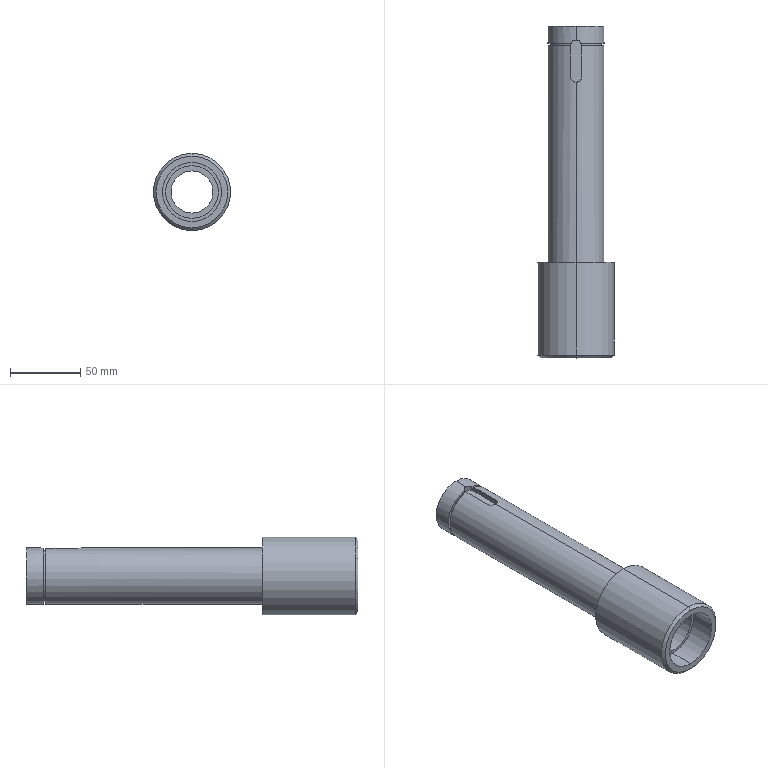Part | SolidWorks | features BaseBody 1 | 1 solid | 37 faces | box 55 x 236 x 55 mm | volume 172352 mm3 | cylinder 22 | plane 13 | cone 2 | commonest cylinder face diameters 40 x6 37.376 x4 8 x2 30 x2 36.4 x2 37 x2
STEP:
#1=CARTESIAN_POINT('',(4.,200.,19.596));
#2=VERTEX_POINT('',#1);
#3=CARTESIAN_POINT('',(0.,196.,20.));
#4=VERTEX_POINT('',#3);
#5=CARTESIAN_POINT('',(4.,200.,19.596));
#6=CARTESIAN_POINT('',(4.,199.735,19.596));
#7=CARTESIAN_POINT('',(3.974,199.475,19.601));
#8=CARTESIAN_POINT('',(3.872,198.963,19.622));
#9=CARTESIAN_POINT('',(3.795,198.709,19.637));
#10=CARTESIAN_POINT('',(3.594,198.225,19.675));
#11=CARTESIAN_POINT('',(3.471,197.996,19.697));
#12=CARTESIAN_POINT('',(3.181,197.561,19.746));
#13=CARTESIAN_POINT('',(3.013,197.356,19.773));
#14=CARTESIAN_POINT('',(2.645,196.989,19.825));
#15=CARTESIAN_POINT('',(2.445,196.823,19.851));
#16=CARTESIAN_POINT('',(2.008,196.531,19.9));
#17=CARTESIAN_POINT('',(1.777,196.407,19.922));
#18=CARTESIAN_POINT('',(1.296,196.207,19.959));
#19=CARTESIAN_POINT('',(1.044,196.13,19.974));
#20=CARTESIAN_POINT('',(0.5265,196.026,19.995));
#21=CARTESIAN_POINT('',(0.2648,196.,20.));
#22=CARTESIAN_POINT('',(0.,196.,20.));
#23=B_SPLINE_CURVE_WITH_KNOTS('',3,(#5,#6,#7,#8,#9,#10,#11,#12,#13,#14,#15,#16,#17,#18,#19,#20,#21,#22),.UNSPECIFIED.,.F.,.F.,(4,2,2,2,2,2,2,2,4),(0.,0.0007831,0.001566,0.002349,0.003132,0.003915,0.004698,0.005481,0.006264),.UNSPECIFIED.);
#24=EDGE_CURVE('',#2,#4,#23,.T.);
#25=ORIENTED_EDGE('',*,*,#24,.T.);
#26=CARTESIAN_POINT('',(0.,68.,20.));
#27=VERTEX_POINT('',#26);
#28=CARTESIAN_POINT('',(0.,236.,20.));
#29=DIRECTION('',(0.,-1.,0.));
#30=VECTOR('',#29,1000.);
#31=LINE('',#28,#30);
#32=EDGE_CURVE('',#4,#27,#31,.T.);
#33=ORIENTED_EDGE('',*,*,#32,.T.);
#34=CARTESIAN_POINT('',(0.,68.,-20.));
#35=VERTEX_POINT('',#34);
#36=CARTESIAN_POINT('',(0.,68.,0.));
#37=DIRECTION('',(0.,1.,0.));
#38=DIRECTION('',(0.,0.,-1.));
#39=AXIS2_PLACEMENT_3D('',#36,#37,#38);
#40=CIRCLE('',#39,20.);
#41=EDGE_CURVE('',#27,#35,#40,.T.);
#42=ORIENTED_EDGE('',*,*,#41,.T.);
#43=CARTESIAN_POINT('',(0.,222.,-20.));
#44=VERTEX_POINT('',#43);
#45=CARTESIAN_POINT('',(0.,236.,-20.));
#46=DIRECTION('',(0.,-1.,0.));
#47=VECTOR('',#46,1000.);
#48=LINE('',#45,#47);
#49=EDGE_CURVE('',#44,#35,#48,.T.);
#50=ORIENTED_EDGE('',*,*,#49,.F.);
#51=CARTESIAN_POINT('',(4.,222.,19.596));
#52=VERTEX_POINT('',#51);
#53=CARTESIAN_POINT('',(0.,222.,0.));
#54=DIRECTION('',(0.,-1.,0.));
#55=DIRECTION('',(0.,0.,-1.));
#56=AXIS2_PLACEMENT_3D('',#53,#54,#55);
#57=CIRCLE('',#56,20.);
#58=EDGE_CURVE('',#44,#52,#57,.T.);
#59=ORIENTED_EDGE('',*,*,#58,.T.);
#60=CARTESIAN_POINT('',(4.,236.,19.596));
#61=DIRECTION('',(0.,-1.,0.));
#62=VECTOR('',#61,1000.);
#63=LINE('',#60,#62);
#64=EDGE_CURVE('',#52,#2,#63,.T.);
#65=ORIENTED_EDGE('',*,*,#64,.T.);
#66=EDGE_LOOP('',(#25,#33,#42,#50,#59,#65));
#67=FACE_OUTER_BOUND('',#66,.T.);
#68=CARTESIAN_POINT('',(0.,236.,0.));
#69=DIRECTION('',(0.,-1.,0.));
#70=DIRECTION('',(0.,0.,-1.));
#71=AXIS2_PLACEMENT_3D('',#68,#69,#70);
#72=CYLINDRICAL_SURFACE('',#71,20.);
#73=ADVANCED_FACE('',(#67),#72,.T.);
#74=CARTESIAN_POINT('',(-3.666,223.6,17.827));
#75=VERTEX_POINT('',#74);
#76=CARTESIAN_POINT('',(0.,223.6,-18.2));
#77=VERTEX_POINT('',#76);
#78=CARTESIAN_POINT('',(0.,223.6,0.));
#79=DIRECTION('',(0.,-1.,0.));
#80=DIRECTION('',(0.,0.,-1.));
#81=AXIS2_PLACEMENT_3D('',#78,#79,#80);
#82=CIRCLE('',#81,18.2);
#83=EDGE_CURVE('',#75,#77,#82,.T.);
#84=ORIENTED_EDGE('',*,*,#83,.T.);
#85=CARTESIAN_POINT('',(0.,222.,-18.2));
#86=VERTEX_POINT('',#85);
#87=CARTESIAN_POINT('',(0.,223.6,-18.2));
#88=DIRECTION('',(0.,-1.,0.));
#89=VECTOR('',#88,1000.);
#90=LINE('',#87,#89);
#91=EDGE_CURVE('',#77,#86,#90,.T.);
#92=ORIENTED_EDGE('',*,*,#91,.T.);
#93=CARTESIAN_POINT('',(-4.,222.,17.755));
#94=VERTEX_POINT('',#93);
#95=CARTESIAN_POINT('',(0.,222.,0.));
#96=DIRECTION('',(0.,-1.,0.));
#97=DIRECTION('',(0.,0.,-1.));
#98=AXIS2_PLACEMENT_3D('',#95,#96,#97);
#99=CIRCLE('',#98,18.2);
#100=EDGE_CURVE('',#94,#86,#99,.T.);
#101=ORIENTED_EDGE('',*,*,#100,.F.);
#102=CARTESIAN_POINT('',(-4.,222.,17.755));
#103=CARTESIAN_POINT('',(-4.,222.277,17.755));
#104=CARTESIAN_POINT('',(-3.972,222.549,17.761));
#105=CARTESIAN_POINT('',(-3.86,223.083,17.786));
#106=CARTESIAN_POINT('',(-3.776,223.347,17.804));
#107=CARTESIAN_POINT('',(-3.666,223.6,17.827));
#108=B_SPLINE_CURVE_WITH_KNOTS('',3,(#102,#103,#104,#105,#106,#107),.UNSPECIFIED.,.F.,.F.,(4,2,4),(0.,0.0008187,0.001637),.UNSPECIFIED.);
#109=EDGE_CURVE('',#94,#75,#108,.T.);
#110=ORIENTED_EDGE('',*,*,#109,.T.);
#111=EDGE_LOOP('',(#84,#92,#101,#110));
#112=FACE_OUTER_BOUND('',#111,.T.);
#113=CARTESIAN_POINT('',(0.,223.6,0.));
#114=DIRECTION('',(0.,-1.,0.));
#115=DIRECTION('',(0.,0.,-1.));
#116=AXIS2_PLACEMENT_3D('',#113,#114,#115);
#117=CYLINDRICAL_SURFACE('',#116,18.2);
#118=ADVANCED_FACE('',(#112),#117,.T.);
#119=CARTESIAN_POINT('',(0.,68.,27.5));
#120=VERTEX_POINT('',#119);
#121=CARTESIAN_POINT('',(0.,68.,-27.5));
#122=VERTEX_POINT('',#121);
#123=CARTESIAN_POINT('',(0.,68.,0.));
#124=DIRECTION('',(0.,1.,0.));
#125=DIRECTION('',(0.,0.,-1.));
#126=AXIS2_PLACEMENT_3D('',#123,#124,#125);
#127=CIRCLE('',#126,27.5);
#128=EDGE_CURVE('',#120,#122,#127,.T.);
#129=ORIENTED_EDGE('',*,*,#128,.F.);
#130=CARTESIAN_POINT('',(0.,2.,27.5));
#131=VERTEX_POINT('',#130);
#132=CARTESIAN_POINT('',(0.,68.,27.5));
#133=DIRECTION('',(0.,-1.,0.));
#134=VECTOR('',#133,1000.);
#135=LINE('',#132,#134);
#136=EDGE_CURVE('',#120,#131,#135,.T.);
#137=ORIENTED_EDGE('',*,*,#136,.T.);
#138=CARTESIAN_POINT('',(0.,2.,-27.5));
#139=VERTEX_POINT('',#138);
#140=CARTESIAN_POINT('',(0.,2.,0.));
#141=DIRECTION('',(0.,1.,0.));
#142=DIRECTION('',(0.,0.,-1.));
#143=AXIS2_PLACEMENT_3D('',#140,#141,#142);
#144=CIRCLE('',#143,27.5);
#145=EDGE_CURVE('',#131,#139,#144,.T.);
#146=ORIENTED_EDGE('',*,*,#145,.T.);
#147=CARTESIAN_POINT('',(0.,68.,-27.5));
#148=DIRECTION('',(0.,-1.,0.));
#149=VECTOR('',#148,1000.);
#150=LINE('',#147,#149);
#151=EDGE_CURVE('',#122,#139,#150,.T.);
#152=ORIENTED_EDGE('',*,*,#151,.F.);
#153=EDGE_LOOP('',(#129,#137,#146,#152));
#154=FACE_OUTER_BOUND('',#153,.T.);
#155=CARTESIAN_POINT('',(0.,68.,0.));
#156=DIRECTION('',(0.,-1.,0.));
#157=DIRECTION('',(0.,0.,-1.));
#158=AXIS2_PLACEMENT_3D('',#155,#156,#157);
#159=CYLINDRICAL_SURFACE('',#158,27.5);
#160=ADVANCED_FACE('',(#154),#159,.T.);
#161=CARTESIAN_POINT('',(0.,236.,-20.));
#162=VERTEX_POINT('',#161);
#163=CARTESIAN_POINT('',(0.,236.,20.));
#164=VERTEX_POINT('',#163);
#165=CARTESIAN_POINT('',(0.,236.,0.));
#166=DIRECTION('',(0.,-1.,0.));
#167=DIRECTION('',(0.,0.,-1.));
#168=AXIS2_PLACEMENT_3D('',#165,#166,#167);
#169=CIRCLE('',#168,20.);
#170=EDGE_CURVE('',#162,#164,#169,.T.);
#171=ORIENTED_EDGE('',*,*,#170,.T.);
#172=CARTESIAN_POINT('',(0.,226.,20.));
#173=VERTEX_POINT('',#172);
#174=CARTESIAN_POINT('',(0.,236.,20.));
#175=DIRECTION('',(0.,-1.,0.));
#176=VECTOR('',#175,1000.);
#177=LINE('',#174,#176);
#178=EDGE_CURVE('',#164,#173,#177,.T.);
#179=ORIENTED_EDGE('',*,*,#178,.T.);
#180=CARTESIAN_POINT('',(3.666,223.6,19.661));
#181=VERTEX_POINT('',#180);
#182=CARTESIAN_POINT('',(0.,226.,20.));
#183=CARTESIAN_POINT('',(0.391,226.,20.));
#184=CARTESIAN_POINT('',(0.7721,225.944,19.989));
#185=CARTESIAN_POINT('',(1.33,225.778,19.957));
#186=CARTESIAN_POINT('',(1.513,225.708,19.943));
#187=CARTESIAN_POINT('',(1.862,225.546,19.914));
#188=CARTESIAN_POINT('',(2.03,225.452,19.897));
#189=CARTESIAN_POINT('',(2.352,225.241,19.862));
#190=CARTESIAN_POINT('',(2.507,225.123,19.843));
#191=CARTESIAN_POINT('',(2.796,224.867,19.804));
#192=CARTESIAN_POINT('',(2.93,224.73,19.785));
#193=CARTESIAN_POINT('',(3.302,224.29,19.727));
#194=CARTESIAN_POINT('',(3.51,223.957,19.69));
#195=CARTESIAN_POINT('',(3.666,223.6,19.661));
#196=B_SPLINE_CURVE_WITH_KNOTS('',3,(#182,#183,#184,#185,#186,#187,#188,#189,#190,#191,#192,#193,#194,#195),.UNSPECIFIED.,.F.,.F.,(4,2,2,2,2,2,4),(0.,0.001156,0.001734,0.002312,0.00289,0.003468,0.004624),.UNSPECIFIED.);
#197=EDGE_CURVE('',#173,#181,#196,.T.);
#198=ORIENTED_EDGE('',*,*,#197,.T.);
#199=CARTESIAN_POINT('',(0.,223.6,-20.));
#200=VERTEX_POINT('',#199);
#201=CARTESIAN_POINT('',(0.,223.6,0.));
#202=DIRECTION('',(0.,1.,0.));
#203=DIRECTION('',(0.,0.,-1.));
#204=AXIS2_PLACEMENT_3D('',#201,#202,#203);
#205=CIRCLE('',#204,20.);
#206=EDGE_CURVE('',#181,#200,#205,.T.);
#207=ORIENTED_EDGE('',*,*,#206,.T.);
#208=CARTESIAN_POINT('',(0.,236.,-20.));
#209=DIRECTION('',(0.,-1.,0.));
#210=VECTOR('',#209,1000.);
#211=LINE('',#208,#210);
#212=EDGE_CURVE('',#162,#200,#211,.T.);
#213=ORIENTED_EDGE('',*,*,#212,.F.);
#214=EDGE_LOOP('',(#171,#179,#198,#207,#213));
#215=FACE_OUTER_BOUND('',#214,.T.);
#216=CARTESIAN_POINT('',(0.,236.,0.));
#217=DIRECTION('',(0.,-1.,0.));
#218=DIRECTION('',(0.,0.,-1.));
#219=AXIS2_PLACEMENT_3D('',#216,#217,#218);
#220=CYLINDRICAL_SURFACE('',#219,20.);
#221=ADVANCED_FACE('',(#215),#220,.T.);
#222=CARTESIAN_POINT('',(0.,0.,25.5));
#223=VERTEX_POINT('',#222);
#224=CARTESIAN_POINT('',(0.,0.,-25.5));
#225=VERTEX_POINT('',#224);
#226=CARTESIAN_POINT('',(0.,0.,0.));
#227=DIRECTION('',(0.,1.,0.));
#228=DIRECTION('',(0.,0.,1.));
#229=AXIS2_PLACEMENT_3D('',#226,#227,#228);
#230=CIRCLE('',#229,25.5);
#231=EDGE_CURVE('',#223,#225,#230,.T.);
#232=ORIENTED_EDGE('',*,*,#231,.T.);
#233=CARTESIAN_POINT('',(0.,2.,-27.5));
#234=DIRECTION('',(0.,0.7071,-0.7071));
#235=VECTOR('',#234,1000.);
#236=LINE('',#233,#235);
#237=EDGE_CURVE('',#225,#139,#236,.T.);
#238=ORIENTED_EDGE('',*,*,#237,.T.);
#239=ORIENTED_EDGE('',*,*,#145,.F.);
#240=CARTESIAN_POINT('',(0.,2.,27.5));
#241=DIRECTION('',(0.,0.7071,0.7071));
#242=VECTOR('',#241,1000.);
#243=LINE('',#240,#242);
#244=EDGE_CURVE('',#223,#131,#243,.T.);
#245=ORIENTED_EDGE('',*,*,#244,.F.);
#246=EDGE_LOOP('',(#232,#238,#239,#245));
#247=FACE_OUTER_BOUND('',#246,.T.);
#248=CARTESIAN_POINT('',(0.,2.,0.));
#249=DIRECTION('',(0.,1.,0.));
#250=DIRECTION('',(0.,0.,1.));
#251=AXIS2_PLACEMENT_3D('',#248,#249,#250);
#252=CONICAL_SURFACE('',#251,27.5,0.7854);
#253=ADVANCED_FACE('',(#247),#252,.T.);
#254=CARTESIAN_POINT('',(0.,226.5,-18.5));
#255=VERTEX_POINT('',#254);
#256=CARTESIAN_POINT('',(0.,226.5,18.5));
#257=VERTEX_POINT('',#256);
#258=CARTESIAN_POINT('',(0.,226.5,0.));
#259=DIRECTION('',(0.,1.,0.));
#260=DIRECTION('',(0.,0.,1.));
#261=AXIS2_PLACEMENT_3D('',#258,#259,#260);
#262=CIRCLE('',#261,18.5);
#263=EDGE_CURVE('',#255,#257,#262,.T.);
#264=ORIENTED_EDGE('',*,*,#263,.F.);
#265=CARTESIAN_POINT('',(0.,236.,-18.5));
#266=VERTEX_POINT('',#265);
#267=CARTESIAN_POINT('',(0.,226.5,-18.5));
#268=DIRECTION('',(0.,1.,0.));
#269=VECTOR('',#268,1000.);
#270=LINE('',#267,#269);
#271=EDGE_CURVE('',#255,#266,#270,.T.);
#272=ORIENTED_EDGE('',*,*,#271,.T.);
#273=CARTESIAN_POINT('',(0.,236.,18.5));
#274=VERTEX_POINT('',#273);
#275=CARTESIAN_POINT('',(0.,236.,0.));
#276=DIRECTION('',(0.,-1.,0.));
#277=DIRECTION('',(0.,0.,1.));
#278=AXIS2_PLACEMENT_3D('',#275,#276,#277);
#279=CIRCLE('',#278,18.5);
#280=EDGE_CURVE('',#274,#266,#279,.T.);
#281=ORIENTED_EDGE('',*,*,#280,.F.);
#282=CARTESIAN_POINT('',(0.,226.5,18.5));
#283=DIRECTION('',(0.,1.,0.));
#284=VECTOR('',#283,1000.);
#285=LINE('',#282,#284);
#286=EDGE_CURVE('',#257,#274,#285,.T.);
#287=ORIENTED_EDGE('',*,*,#286,.F.);
#288=EDGE_LOOP('',(#264,#272,#281,#287));
#289=FACE_OUTER_BOUND('',#288,.T.);
#290=CARTESIAN_POINT('',(0.,226.5,0.));
#291=DIRECTION('',(0.,1.,0.));
#292=DIRECTION('',(0.,0.,1.));
#293=AXIS2_PLACEMENT_3D('',#290,#291,#292);
#294=CYLINDRICAL_SURFACE('',#293,18.5);
#295=ADVANCED_FACE('',(#289),#294,.F.);
#296=CARTESIAN_POINT('',(0.,18.,21.));
#297=VERTEX_POINT('',#296);
#298=CARTESIAN_POINT('',(0.,18.,-21.));
#299=VERTEX_POINT('',#298);
#300=CARTESIAN_POINT('',(0.,18.,0.));
#301=DIRECTION('',(0.,-1.,0.));
#302=DIRECTION('',(0.,0.,-1.));
#303=AXIS2_PLACEMENT_3D('',#300,#301,#302);
#304=CIRCLE('',#303,21.);
#305=EDGE_CURVE('',#297,#299,#304,.T.);
#306=ORIENTED_EDGE('',*,*,#305,.F.);
#307=CARTESIAN_POINT('',(0.,0.,21.));
#308=VERTEX_POINT('',#307);
#309=CARTESIAN_POINT('',(0.,18.,21.));
#310=DIRECTION('',(0.,-1.,0.));
#311=VECTOR('',#310,1000.);
#312=LINE('',#309,#311);
#313=EDGE_CURVE('',#297,#308,#312,.T.);
#314=ORIENTED_EDGE('',*,*,#313,.T.);
#315=CARTESIAN_POINT('',(0.,0.,-21.));
#316=VERTEX_POINT('',#315);
#317=CARTESIAN_POINT('',(0.,0.,0.));
#318=DIRECTION('',(0.,-1.,0.));
#319=DIRECTION('',(0.,0.,-1.));
#320=AXIS2_PLACEMENT_3D('',#317,#318,#319);
#321=CIRCLE('',#320,21.);
#322=EDGE_CURVE('',#308,#316,#321,.T.);
#323=ORIENTED_EDGE('',*,*,#322,.T.);
#324=CARTESIAN_POINT('',(0.,18.,-21.));
#325=DIRECTION('',(0.,-1.,0.));
#326=VECTOR('',#325,1000.);
#327=LINE('',#324,#326);
#328=EDGE_CURVE('',#299,#316,#327,.T.);
#329=ORIENTED_EDGE('',*,*,#328,.F.);
#330=EDGE_LOOP('',(#306,#314,#323,#329));
#331=FACE_OUTER_BOUND('',#330,.T.);
#332=CARTESIAN_POINT('',(0.,18.,0.));
#333=DIRECTION('',(0.,-1.,0.));
#334=DIRECTION('',(0.,0.,-1.));
#335=AXIS2_PLACEMENT_3D('',#332,#333,#334);
#336=CYLINDRICAL_SURFACE('',#335,21.);
#337=ADVANCED_FACE('',(#331),#336,.F.);
#338=CARTESIAN_POINT('',(0.,226.5,15.));
#339=VERTEX_POINT('',#338);
#340=CARTESIAN_POINT('',(0.,226.5,-15.));
#341=VERTEX_POINT('',#340);
#342=CARTESIAN_POINT('',(0.,226.5,0.));
#343=DIRECTION('',(0.,-1.,0.));
#344=DIRECTION('',(0.,0.,-1.));
#345=AXIS2_PLACEMENT_3D('',#342,#343,#344);
#346=CIRCLE('',#345,15.);
#347=EDGE_CURVE('',#339,#341,#346,.T.);
#348=ORIENTED_EDGE('',*,*,#347,.F.);
#349=CARTESIAN_POINT('',(0.,58.,15.));
#350=VERTEX_POINT('',#349);
#351=CARTESIAN_POINT('',(0.,68.,15.));
#352=DIRECTION('',(0.,-1.,0.));
#353=VECTOR('',#352,1000.);
#354=LINE('',#351,#353);
#355=EDGE_CURVE('',#339,#350,#354,.T.);
#356=ORIENTED_EDGE('',*,*,#355,.T.);
#357=CARTESIAN_POINT('',(0.,58.,-15.));
#358=VERTEX_POINT('',#357);
#359=CARTESIAN_POINT('',(0.,58.,0.));
#360=DIRECTION('',(0.,1.,0.));
#361=DIRECTION('',(0.,0.,-1.));
#362=AXIS2_PLACEMENT_3D('',#359,#360,#361);
#363=CIRCLE('',#362,15.);
#364=EDGE_CURVE('',#358,#350,#363,.T.);
#365=ORIENTED_EDGE('',*,*,#364,.F.);
#366=CARTESIAN_POINT('',(0.,68.,-15.));
#367=DIRECTION('',(0.,-1.,0.));
#368=VECTOR('',#367,1000.);
#369=LINE('',#366,#368);
#370=EDGE_CURVE('',#341,#358,#369,.T.);
#371=ORIENTED_EDGE('',*,*,#370,.F.);
#372=EDGE_LOOP('',(#348,#356,#365,#371));
#373=FACE_OUTER_BOUND('',#372,.T.);
#374=CARTESIAN_POINT('',(0.,68.,0.));
#375=DIRECTION('',(0.,-1.,0.));
#376=DIRECTION('',(0.,0.,-1.));
#377=AXIS2_PLACEMENT_3D('',#374,#375,#376);
#378=CYLINDRICAL_SURFACE('',#377,15.);
#379=ADVANCED_FACE('',(#373),#378,.F.);
#380=CARTESIAN_POINT('',(0.,48.,18.688));
#381=VERTEX_POINT('',#380);
#382=CARTESIAN_POINT('',(0.,48.,-18.688));
#383=VERTEX_POINT('',#382);
#384=CARTESIAN_POINT('',(0.,48.,0.));
#385=DIRECTION('',(0.,-1.,0.));
#386=DIRECTION('',(0.,0.,-1.));
#387=AXIS2_PLACEMENT_3D('',#384,#385,#386);
#388=CIRCLE('',#387,18.688);
#389=EDGE_CURVE('',#381,#383,#388,.T.);
#390=ORIENTED_EDGE('',*,*,#389,.F.);
#391=CARTESIAN_POINT('',(0.,18.,18.688));
#392=VERTEX_POINT('',#391);
#393=CARTESIAN_POINT('',(0.,58.,18.688));
#394=DIRECTION('',(0.,-1.,0.));
#395=VECTOR('',#394,1000.);
#396=LINE('',#393,#395);
#397=EDGE_CURVE('',#381,#392,#396,.T.);
#398=ORIENTED_EDGE('',*,*,#397,.T.);
#399=CARTESIAN_POINT('',(0.,18.,-18.688));
#400=VERTEX_POINT('',#399);
#401=CARTESIAN_POINT('',(0.,18.,0.));
#402=DIRECTION('',(0.,1.,0.));
#403=DIRECTION('',(0.,0.,-1.));
#404=AXIS2_PLACEMENT_3D('',#401,#402,#403);
#405=CIRCLE('',#404,18.688);
#406=EDGE_CURVE('',#400,#392,#405,.T.);
#407=ORIENTED_EDGE('',*,*,#406,.F.);
#408=CARTESIAN_POINT('',(0.,58.,-18.688));
#409=DIRECTION('',(0.,-1.,0.));
#410=VECTOR('',#409,1000.);
#411=LINE('',#408,#410);
#412=EDGE_CURVE('',#383,#400,#411,.T.);
#413=ORIENTED_EDGE('',*,*,#412,.F.);
#414=EDGE_LOOP('',(#390,#398,#407,#413));
#415=FACE_OUTER_BOUND('',#414,.T.);
#416=CARTESIAN_POINT('',(0.,58.,0.));
#417=DIRECTION('',(0.,-1.,0.));
#418=DIRECTION('',(0.,0.,-1.));
#419=AXIS2_PLACEMENT_3D('',#416,#417,#418);
#420=CYLINDRICAL_SURFACE('',#419,18.688);
#421=ADVANCED_FACE('',(#415),#420,.F.);
#422=CARTESIAN_POINT('',(0.,58.,18.688));
#423=VERTEX_POINT('',#422);
#424=CARTESIAN_POINT('',(0.,58.,-18.688));
#425=VERTEX_POINT('',#424);
#426=CARTESIAN_POINT('',(0.,58.,0.));
#427=DIRECTION('',(0.,-1.,0.));
#428=DIRECTION('',(0.,0.,-1.));
#429=AXIS2_PLACEMENT_3D('',#426,#427,#428);
#430=CIRCLE('',#429,18.688);
#431=EDGE_CURVE('',#423,#425,#430,.T.);
#432=ORIENTED_EDGE('',*,*,#431,.F.);
#433=CARTESIAN_POINT('',(0.,52.,18.688));
#434=VERTEX_POINT('',#433);
#435=CARTESIAN_POINT('',(0.,58.,18.688));
#436=DIRECTION('',(0.,-1.,0.));
#437=VECTOR('',#436,1000.);
#438=LINE('',#435,#437);
#439=EDGE_CURVE('',#423,#434,#438,.T.);
#440=ORIENTED_EDGE('',*,*,#439,.T.);
#441=CARTESIAN_POINT('',(0.,52.,-18.688));
#442=VERTEX_POINT('',#441);
#443=CARTESIAN_POINT('',(0.,52.,0.));
#444=DIRECTION('',(0.,1.,0.));
#445=DIRECTION('',(0.,0.,-1.));
#446=AXIS2_PLACEMENT_3D('',#443,#444,#445);
#447=CIRCLE('',#446,18.688);
#448=EDGE_CURVE('',#442,#434,#447,.T.);
#449=ORIENTED_EDGE('',*,*,#448,.F.);
#450=CARTESIAN_POINT('',(0.,58.,-18.688));
#451=DIRECTION('',(0.,-1.,0.));
#452=VECTOR('',#451,1000.);
#453=LINE('',#450,#452);
#454=EDGE_CURVE('',#425,#442,#453,.T.);
#455=ORIENTED_EDGE('',*,*,#454,.F.);
#456=EDGE_LOOP('',(#432,#440,#449,#455));
#457=FACE_OUTER_BOUND('',#456,.T.);
#458=CARTESIAN_POINT('',(0.,58.,0.));
#459=DIRECTION('',(0.,-1.,0.));
#460=DIRECTION('',(0.,0.,-1.));
#461=AXIS2_PLACEMENT_3D('',#458,#459,#460);
#462=CYLINDRICAL_SURFACE('',#461,18.688);
#463=ADVANCED_FACE('',(#457),#462,.F.);
#464=CARTESIAN_POINT('',(0.,52.,20.));
#465=VERTEX_POINT('',#464);
#466=CARTESIAN_POINT('',(0.,52.,-20.));
#467=VERTEX_POINT('',#466);
#468=CARTESIAN_POINT('',(0.,52.,0.));
#469=DIRECTION('',(0.,-1.,0.));
#470=DIRECTION('',(0.,0.,-1.));
#471=AXIS2_PLACEMENT_3D('',#468,#469,#470);
#472=CIRCLE('',#471,20.);
#473=EDGE_CURVE('',#465,#467,#472,.T.);
#474=ORIENTED_EDGE('',*,*,#473,.F.);
#475=CARTESIAN_POINT('',(0.,48.,20.));
#476=VERTEX_POINT('',#475);
#477=CARTESIAN_POINT('',(0.,52.,20.));
#478=DIRECTION('',(0.,-1.,0.));
#479=VECTOR('',#478,1000.);
#480=LINE('',#477,#479);
#481=EDGE_CURVE('',#465,#476,#480,.T.);
#482=ORIENTED_EDGE('',*,*,#481,.T.);
#483=CARTESIAN_POINT('',(0.,48.,-20.));
#484=VERTEX_POINT('',#483);
#485=CARTESIAN_POINT('',(0.,48.,0.));
#486=DIRECTION('',(0.,-1.,0.));
#487=DIRECTION('',(0.,0.,-1.));
#488=AXIS2_PLACEMENT_3D('',#485,#486,#487);
#489=CIRCLE('',#488,20.);
#490=EDGE_CURVE('',#476,#484,#489,.T.);
#491=ORIENTED_EDGE('',*,*,#490,.T.);
#492=CARTESIAN_POINT('',(0.,52.,-20.));
#493=DIRECTION('',(0.,-1.,0.));
#494=VECTOR('',#493,1000.);
#495=LINE('',#492,#494);
#496=EDGE_CURVE('',#467,#484,#495,.T.);
#497=ORIENTED_EDGE('',*,*,#496,.F.);
#498=EDGE_LOOP('',(#474,#482,#491,#497));
#499=FACE_OUTER_BOUND('',#498,.T.);
#500=CARTESIAN_POINT('',(0.,52.,0.));
#501=DIRECTION('',(0.,-1.,0.));
#502=DIRECTION('',(0.,0.,-1.));
#503=AXIS2_PLACEMENT_3D('',#500,#501,#502);
#504=CYLINDRICAL_SURFACE('',#503,20.);
#505=ADVANCED_FACE('',(#499),#504,.F.);
#506=ORIENTED_EDGE('',*,*,#32,.F.);
#507=CARTESIAN_POINT('',(-4.,200.,19.596));
#508=VERTEX_POINT('',#507);
#509=CARTESIAN_POINT('',(0.,196.,20.));
#510=CARTESIAN_POINT('',(-0.2648,196.,20.));
#511=CARTESIAN_POINT('',(-0.5251,196.026,19.995));
#512=CARTESIAN_POINT('',(-1.037,196.128,19.975));
#513=CARTESIAN_POINT('',(-1.291,196.205,19.96));
#514=CARTESIAN_POINT('',(-1.775,196.406,19.923));
#515=CARTESIAN_POINT('',(-2.005,196.529,19.9));
#516=CARTESIAN_POINT('',(-2.439,196.819,19.852));
#517=CARTESIAN_POINT('',(-2.644,196.987,19.825));
#518=CARTESIAN_POINT('',(-3.012,197.355,19.773));
#519=CARTESIAN_POINT('',(-3.177,197.555,19.747));
#520=CARTESIAN_POINT('',(-3.469,197.992,19.697));
#521=CARTESIAN_POINT('',(-3.593,198.223,19.675));
#522=CARTESIAN_POINT('',(-3.793,198.704,19.637));
#523=CARTESIAN_POINT('',(-3.87,198.956,19.622));
#524=CARTESIAN_POINT('',(-3.974,199.473,19.601));
#525=CARTESIAN_POINT('',(-4.,199.735,19.596));
#526=CARTESIAN_POINT('',(-4.,200.,19.596));
#527=B_SPLINE_CURVE_WITH_KNOTS('',3,(#509,#510,#511,#512,#513,#514,#515,#516,#517,#518,#519,#520,#521,#522,#523,#524,#525,#526),.UNSPECIFIED.,.F.,.F.,(4,2,2,2,2,2,2,2,4),(0.006264,0.007048,0.007831,0.008614,0.009397,0.01018,0.01096,0.01175,0.01253),.UNSPECIFIED.);
#528=EDGE_CURVE('',#4,#508,#527,.T.);
#529=ORIENTED_EDGE('',*,*,#528,.T.);
#530=CARTESIAN_POINT('',(-4.,222.,19.596));
#531=VERTEX_POINT('',#530);
#532=CARTESIAN_POINT('',(-4.,236.,19.596));
#533=DIRECTION('',(0.,1.,0.));
#534=VECTOR('',#533,1000.);
#535=LINE('',#532,#534);
#536=EDGE_CURVE('',#508,#531,#535,.T.);
#537=ORIENTED_EDGE('',*,*,#536,.T.);
#538=CARTESIAN_POINT('',(0.,222.,0.));
#539=DIRECTION('',(0.,-1.,0.));
#540=DIRECTION('',(0.,0.,-1.));
#541=AXIS2_PLACEMENT_3D('',#538,#539,#540);
#542=CIRCLE('',#541,20.);
#543=EDGE_CURVE('',#531,#44,#542,.T.);
#544=ORIENTED_EDGE('',*,*,#543,.T.);
#545=ORIENTED_EDGE('',*,*,#49,.T.);
#546=CARTESIAN_POINT('',(0.,68.,0.));
#547=DIRECTION('',(0.,1.,0.));
#548=DIRECTION('',(0.,0.,-1.));
#549=AXIS2_PLACEMENT_3D('',#546,#547,#548);
#550=CIRCLE('',#549,20.);
#551=EDGE_CURVE('',#35,#27,#550,.T.);
#552=ORIENTED_EDGE('',*,*,#551,.T.);
#553=EDGE_LOOP('',(#506,#529,#537,#544,#545,#552));
#554=FACE_OUTER_BOUND('',#553,.T.);
#555=CARTESIAN_POINT('',(0.,236.,0.));
#556=DIRECTION('',(0.,-1.,0.));
#557=DIRECTION('',(0.,0.,-1.));
#558=AXIS2_PLACEMENT_3D('',#555,#556,#557);
#559=CYLINDRICAL_SURFACE('',#558,20.);
#560=ADVANCED_FACE('',(#554),#559,.T.);
#561=CARTESIAN_POINT('',(4.,200.,16.));
#562=VERTEX_POINT('',#561);
#563=CARTESIAN_POINT('',(4.,222.,16.));
#564=VERTEX_POINT('',#563);
#565=CARTESIAN_POINT('',(4.,222.,16.));
#566=DIRECTION('',(0.,1.,0.));
#567=VECTOR('',#566,1000.);
#568=LINE('',#565,#567);
#569=EDGE_CURVE('',#562,#564,#568,.T.);
#570=ORIENTED_EDGE('',*,*,#569,.F.);
#571=CARTESIAN_POINT('',(4.,200.,16.));
#572=DIRECTION('',(0.,0.,-1.));
#573=VECTOR('',#572,1000.);
#574=LINE('',#571,#573);
#575=EDGE_CURVE('',#2,#562,#574,.T.);
#576=ORIENTED_EDGE('',*,*,#575,.F.);
#577=ORIENTED_EDGE('',*,*,#64,.F.);
#578=CARTESIAN_POINT('',(4.,222.,17.755));
#579=VERTEX_POINT('',#578);
#580=CARTESIAN_POINT('',(4.,222.,16.));
#581=DIRECTION('',(0.,0.,1.));
#582=VECTOR('',#581,1000.);
#583=LINE('',#580,#582);
#584=EDGE_CURVE('',#579,#52,#583,.T.);
#585=ORIENTED_EDGE('',*,*,#584,.F.);
#586=CARTESIAN_POINT('',(4.,222.,16.));
#587=DIRECTION('',(0.,0.,1.));
#588=VECTOR('',#587,1000.);
#589=LINE('',#586,#588);
#590=EDGE_CURVE('',#564,#579,#589,.T.);
#591=ORIENTED_EDGE('',*,*,#590,.F.);
#592=EDGE_LOOP('',(#570,#576,#577,#585,#591));
#593=FACE_OUTER_BOUND('',#592,.T.);
#594=CARTESIAN_POINT('',(4.,222.,16.));
#595=DIRECTION('',(1.,0.,0.));
#596=DIRECTION('',(0.,1.,0.));
#597=AXIS2_PLACEMENT_3D('',#594,#595,#596);
#598=PLANE('',#597);
#599=ADVANCED_FACE('',(#593),#598,.F.);
#600=CARTESIAN_POINT('',(-4.,222.,0.));
#601=DIRECTION('',(0.,0.,-1.));
#602=VECTOR('',#601,1000.);
#603=LINE('',#600,#602);
#604=EDGE_CURVE('',#531,#94,#603,.T.);
#605=ORIENTED_EDGE('',*,*,#604,.T.);
#606=ORIENTED_EDGE('',*,*,#100,.T.);
#607=CARTESIAN_POINT('',(0.,222.,0.));
#608=DIRECTION('',(0.,-1.,0.));
#609=DIRECTION('',(0.,0.,-1.));
#610=AXIS2_PLACEMENT_3D('',#607,#608,#609);
#611=CIRCLE('',#610,18.2);
#612=EDGE_CURVE('',#86,#579,#611,.T.);
#613=ORIENTED_EDGE('',*,*,#612,.T.);
#614=ORIENTED_EDGE('',*,*,#584,.T.);
#615=ORIENTED_EDGE('',*,*,#58,.F.);
#616=ORIENTED_EDGE('',*,*,#543,.F.);
#617=EDGE_LOOP('',(#605,#606,#613,#614,#615,#616));
#618=FACE_OUTER_BOUND('',#617,.T.);
#619=CARTESIAN_POINT('',(0.,222.,0.));
#620=DIRECTION('',(0.,1.,0.));
#621=DIRECTION('',(0.,0.,1.));
#622=AXIS2_PLACEMENT_3D('',#619,#620,#621);
#623=PLANE('',#622);
#624=ADVANCED_FACE('',(#618),#623,.T.);
#625=ORIENTED_EDGE('',*,*,#551,.F.);
#626=ORIENTED_EDGE('',*,*,#41,.F.);
#627=EDGE_LOOP('',(#625,#626));
#628=FACE_BOUND('',#627,.T.);
#629=CARTESIAN_POINT('',(0.,68.,0.));
#630=DIRECTION('',(0.,1.,0.));
#631=DIRECTION('',(0.,0.,-1.));
#632=AXIS2_PLACEMENT_3D('',#629,#630,#631);
#633=CIRCLE('',#632,27.5);
#634=EDGE_CURVE('',#122,#120,#633,.T.);
#635=ORIENTED_EDGE('',*,*,#634,.T.);
#636=ORIENTED_EDGE('',*,*,#128,.T.);
#637=EDGE_LOOP('',(#635,#636));
#638=FACE_OUTER_BOUND('',#637,.T.);
#639=CARTESIAN_POINT('',(0.,68.,0.));
#640=DIRECTION('',(0.,1.,0.));
#641=DIRECTION('',(0.,0.,1.));
#642=AXIS2_PLACEMENT_3D('',#639,#640,#641);
#643=PLANE('',#642);
#644=ADVANCED_FACE('',(#628,#638),#643,.T.);
#645=CARTESIAN_POINT('',(-4.,200.,16.));
#646=VERTEX_POINT('',#645);
#647=CARTESIAN_POINT('',(0.,200.,16.));
#648=DIRECTION('',(0.,0.,1.));
#649=DIRECTION('',(1.,0.,0.));
#650=AXIS2_PLACEMENT_3D('',#647,#648,#649);
#651=CIRCLE('',#650,4.);
#652=EDGE_CURVE('',#646,#562,#651,.T.);
#653=ORIENTED_EDGE('',*,*,#652,.F.);
#654=CARTESIAN_POINT('',(-4.,200.,16.));
#655=DIRECTION('',(0.,0.,-1.));
#656=VECTOR('',#655,1000.);
#657=LINE('',#654,#656);
#658=EDGE_CURVE('',#508,#646,#657,.T.);
#659=ORIENTED_EDGE('',*,*,#658,.F.);
#660=ORIENTED_EDGE('',*,*,#528,.F.);
#661=ORIENTED_EDGE('',*,*,#24,.F.);
#662=ORIENTED_EDGE('',*,*,#575,.T.);
#663=EDGE_LOOP('',(#653,#659,#660,#661,#662));
#664=FACE_OUTER_BOUND('',#663,.T.);
#665=CARTESIAN_POINT('',(0.,200.,16.));
#666=DIRECTION('',(0.,0.,1.));
#667=DIRECTION('',(1.,0.,0.));
#668=AXIS2_PLACEMENT_3D('',#665,#666,#667);
#669=CYLINDRICAL_SURFACE('',#668,4.);
#670=ADVANCED_FACE('',(#664),#669,.F.);
#671=CARTESIAN_POINT('',(3.666,223.6,17.827));
#672=VERTEX_POINT('',#671);
#673=CARTESIAN_POINT('',(3.666,223.6,16.));
#674=DIRECTION('',(0.,0.,-1.));
#675=VECTOR('',#674,1000.);
#676=LINE('',#673,#675);
#677=EDGE_CURVE('',#181,#672,#676,.T.);
#678=ORIENTED_EDGE('',*,*,#677,.F.);
#679=ORIENTED_EDGE('',*,*,#197,.F.);
#680=CARTESIAN_POINT('',(-3.666,223.6,19.661));
#681=VERTEX_POINT('',#680);
#682=CARTESIAN_POINT('',(-3.666,223.6,19.661));
#683=CARTESIAN_POINT('',(-3.51,223.957,19.69));
#684=CARTESIAN_POINT('',(-3.307,224.283,19.726));
#685=CARTESIAN_POINT('',(-2.934,224.726,19.784));
#686=CARTESIAN_POINT('',(-2.797,224.866,19.804));
#687=CARTESIAN_POINT('',(-2.509,225.121,19.842));
#688=CARTESIAN_POINT('',(-2.357,225.237,19.861));
#689=CARTESIAN_POINT('',(-2.035,225.449,19.897));
#690=CARTESIAN_POINT('',(-1.865,225.544,19.914));
#691=CARTESIAN_POINT('',(-1.514,225.708,19.943));
#692=CARTESIAN_POINT('',(-1.334,225.776,19.956));
#693=CARTESIAN_POINT('',(-0.781,225.942,19.988));
#694=CARTESIAN_POINT('',(-0.3911,226.,20.));
#695=CARTESIAN_POINT('',(0.,226.,20.));
#696=B_SPLINE_CURVE_WITH_KNOTS('',3,(#682,#683,#684,#685,#686,#687,#688,#689,#690,#691,#692,#693,#694,#695),.UNSPECIFIED.,.F.,.F.,(4,2,2,2,2,2,4),(-0.004625,-0.003469,-0.002891,-0.002313,-0.001735,-0.001156,0.),.UNSPECIFIED.);
#697=EDGE_CURVE('',#681,#173,#696,.T.);
#698=ORIENTED_EDGE('',*,*,#697,.F.);
#699=CARTESIAN_POINT('',(-3.666,223.6,16.));
#700=DIRECTION('',(0.,0.,1.));
#701=VECTOR('',#700,1000.);
#702=LINE('',#699,#701);
#703=EDGE_CURVE('',#75,#681,#702,.T.);
#704=ORIENTED_EDGE('',*,*,#703,.F.);
#705=ORIENTED_EDGE('',*,*,#109,.F.);
#706=CARTESIAN_POINT('',(-4.,222.,16.));
#707=VERTEX_POINT('',#706);
#708=CARTESIAN_POINT('',(-4.,222.,16.));
#709=DIRECTION('',(0.,0.,1.));
#710=VECTOR('',#709,1000.);
#711=LINE('',#708,#710);
#712=EDGE_CURVE('',#707,#94,#711,.T.);
#713=ORIENTED_EDGE('',*,*,#712,.F.);
#714=CARTESIAN_POINT('',(0.,222.,16.));
#715=DIRECTION('',(0.,0.,1.));
#716=DIRECTION('',(1.,0.,0.));
#717=AXIS2_PLACEMENT_3D('',#714,#715,#716);
#718=CIRCLE('',#717,4.);
#719=EDGE_CURVE('',#564,#707,#718,.T.);
#720=ORIENTED_EDGE('',*,*,#719,.F.);
#721=ORIENTED_EDGE('',*,*,#590,.T.);
#722=CARTESIAN_POINT('',(3.666,223.6,17.827));
#723=CARTESIAN_POINT('',(3.776,223.347,17.804));
#724=CARTESIAN_POINT('',(3.859,223.087,17.786));
#725=CARTESIAN_POINT('',(3.971,222.553,17.762));
#726=CARTESIAN_POINT('',(4.,222.277,17.755));
#727=CARTESIAN_POINT('',(4.,222.,17.755));
#728=B_SPLINE_CURVE_WITH_KNOTS('',3,(#722,#723,#724,#725,#726,#727),.UNSPECIFIED.,.F.,.F.,(4,2,4),(0.,0.0008187,0.001637),.UNSPECIFIED.);
#729=EDGE_CURVE('',#672,#579,#728,.T.);
#730=ORIENTED_EDGE('',*,*,#729,.F.);
#731=EDGE_LOOP('',(#678,#679,#698,#704,#705,#713,#720,#721,#730));
#732=FACE_OUTER_BOUND('',#731,.T.);
#733=CARTESIAN_POINT('',(0.,222.,16.));
#734=DIRECTION('',(0.,0.,1.));
#735=DIRECTION('',(1.,0.,0.));
#736=AXIS2_PLACEMENT_3D('',#733,#734,#735);
#737=CYLINDRICAL_SURFACE('',#736,4.);
#738=ADVANCED_FACE('',(#732),#737,.F.);
#739=ORIENTED_EDGE('',*,*,#652,.T.);
#740=ORIENTED_EDGE('',*,*,#569,.T.);
#741=ORIENTED_EDGE('',*,*,#719,.T.);
#742=CARTESIAN_POINT('',(-4.,222.,16.));
#743=DIRECTION('',(0.,-1.,0.));
#744=VECTOR('',#743,1000.);
#745=LINE('',#742,#744);
#746=EDGE_CURVE('',#707,#646,#745,.T.);
#747=ORIENTED_EDGE('',*,*,#746,.T.);
#748=EDGE_LOOP('',(#739,#740,#741,#747));
#749=FACE_OUTER_BOUND('',#748,.T.);
#750=CARTESIAN_POINT('',(0.,222.,16.));
#751=DIRECTION('',(0.,0.,1.));
#752=DIRECTION('',(1.,0.,0.));
#753=AXIS2_PLACEMENT_3D('',#750,#751,#752);
#754=PLANE('',#753);
#755=ADVANCED_FACE('',(#749),#754,.T.);
#756=ORIENTED_EDGE('',*,*,#91,.F.);
#757=CARTESIAN_POINT('',(0.,223.6,0.));
#758=DIRECTION('',(0.,-1.,0.));
#759=DIRECTION('',(0.,0.,-1.));
#760=AXIS2_PLACEMENT_3D('',#757,#758,#759);
#761=CIRCLE('',#760,18.2);
#762=EDGE_CURVE('',#77,#672,#761,.T.);
#763=ORIENTED_EDGE('',*,*,#762,.T.);
#764=ORIENTED_EDGE('',*,*,#729,.T.);
#765=ORIENTED_EDGE('',*,*,#612,.F.);
#766=EDGE_LOOP('',(#756,#763,#764,#765));
#767=FACE_OUTER_BOUND('',#766,.T.);
#768=CARTESIAN_POINT('',(0.,223.6,0.));
#769=DIRECTION('',(0.,-1.,0.));
#770=DIRECTION('',(0.,0.,-1.));
#771=AXIS2_PLACEMENT_3D('',#768,#769,#770);
#772=CYLINDRICAL_SURFACE('',#771,18.2);
#773=ADVANCED_FACE('',(#767),#772,.T.);
#774=ORIENTED_EDGE('',*,*,#746,.F.);
#775=ORIENTED_EDGE('',*,*,#712,.T.);
#776=ORIENTED_EDGE('',*,*,#604,.F.);
#777=ORIENTED_EDGE('',*,*,#536,.F.);
#778=ORIENTED_EDGE('',*,*,#658,.T.);
#779=EDGE_LOOP('',(#774,#775,#776,#777,#778));
#780=FACE_OUTER_BOUND('',#779,.T.);
#781=CARTESIAN_POINT('',(-4.,222.,16.));
#782=DIRECTION('',(-1.,0.,0.));
#783=DIRECTION('',(0.,-1.,0.));
#784=AXIS2_PLACEMENT_3D('',#781,#782,#783);
#785=PLANE('',#784);
#786=ADVANCED_FACE('',(#780),#785,.F.);
#787=ORIENTED_EDGE('',*,*,#136,.F.);
#788=ORIENTED_EDGE('',*,*,#634,.F.);
#789=ORIENTED_EDGE('',*,*,#151,.T.);
#790=CARTESIAN_POINT('',(0.,2.,0.));
#791=DIRECTION('',(0.,1.,0.));
#792=DIRECTION('',(0.,0.,-1.));
#793=AXIS2_PLACEMENT_3D('',#790,#791,#792);
#794=CIRCLE('',#793,27.5);
#795=EDGE_CURVE('',#139,#131,#794,.T.);
#796=ORIENTED_EDGE('',*,*,#795,.T.);
#797=EDGE_LOOP('',(#787,#788,#789,#796));
#798=FACE_OUTER_BOUND('',#797,.T.);
#799=CARTESIAN_POINT('',(0.,68.,0.));
#800=DIRECTION('',(0.,-1.,0.));
#801=DIRECTION('',(0.,0.,-1.));
#802=AXIS2_PLACEMENT_3D('',#799,#800,#801);
#803=CYLINDRICAL_SURFACE('',#802,27.5);
#804=ADVANCED_FACE('',(#798),#803,.T.);
#805=ORIENTED_EDGE('',*,*,#677,.T.);
#806=ORIENTED_EDGE('',*,*,#762,.F.);
#807=ORIENTED_EDGE('',*,*,#83,.F.);
#808=ORIENTED_EDGE('',*,*,#703,.T.);
#809=CARTESIAN_POINT('',(0.,223.6,0.));
#810=DIRECTION('',(0.,1.,0.));
#811=DIRECTION('',(0.,0.,-1.));
#812=AXIS2_PLACEMENT_3D('',#809,#810,#811);
#813=CIRCLE('',#812,20.);
#814=EDGE_CURVE('',#200,#681,#813,.T.);
#815=ORIENTED_EDGE('',*,*,#814,.F.);
#816=ORIENTED_EDGE('',*,*,#206,.F.);
#817=EDGE_LOOP('',(#805,#806,#807,#808,#815,#816));
#818=FACE_OUTER_BOUND('',#817,.T.);
#819=CARTESIAN_POINT('',(0.,223.6,0.));
#820=DIRECTION('',(0.,1.,0.));
#821=DIRECTION('',(0.,0.,1.));
#822=AXIS2_PLACEMENT_3D('',#819,#820,#821);
#823=PLANE('',#822);
#824=ADVANCED_FACE('',(#818),#823,.F.);
#825=ORIENTED_EDGE('',*,*,#178,.F.);
#826=CARTESIAN_POINT('',(0.,236.,0.));
#827=DIRECTION('',(0.,-1.,0.));
#828=DIRECTION('',(0.,0.,-1.));
#829=AXIS2_PLACEMENT_3D('',#826,#827,#828);
#830=CIRCLE('',#829,20.);
#831=EDGE_CURVE('',#164,#162,#830,.T.);
#832=ORIENTED_EDGE('',*,*,#831,.T.);
#833=ORIENTED_EDGE('',*,*,#212,.T.);
#834=ORIENTED_EDGE('',*,*,#814,.T.);
#835=ORIENTED_EDGE('',*,*,#697,.T.);
#836=EDGE_LOOP('',(#825,#832,#833,#834,#835));
#837=FACE_OUTER_BOUND('',#836,.T.);
#838=CARTESIAN_POINT('',(0.,236.,0.));
#839=DIRECTION('',(0.,-1.,0.));
#840=DIRECTION('',(0.,0.,-1.));
#841=AXIS2_PLACEMENT_3D('',#838,#839,#840);
#842=CYLINDRICAL_SURFACE('',#841,20.);
#843=ADVANCED_FACE('',(#837),#842,.T.);
#844=ORIENTED_EDGE('',*,*,#237,.F.);
#845=CARTESIAN_POINT('',(0.,0.,0.));
#846=DIRECTION('',(0.,1.,0.));
#847=DIRECTION('',(0.,0.,1.));
#848=AXIS2_PLACEMENT_3D('',#845,#846,#847);
#849=CIRCLE('',#848,25.5);
#850=EDGE_CURVE('',#225,#223,#849,.T.);
#851=ORIENTED_EDGE('',*,*,#850,.T.);
#852=ORIENTED_EDGE('',*,*,#244,.T.);
#853=ORIENTED_EDGE('',*,*,#795,.F.);
#854=EDGE_LOOP('',(#844,#851,#852,#853));
#855=FACE_OUTER_BOUND('',#854,.T.);
#856=CARTESIAN_POINT('',(0.,2.,0.));
#857=DIRECTION('',(0.,1.,0.));
#858=DIRECTION('',(0.,0.,1.));
#859=AXIS2_PLACEMENT_3D('',#856,#857,#858);
#860=CONICAL_SURFACE('',#859,27.5,0.7854);
#861=ADVANCED_FACE('',(#855),#860,.T.);
#862=ORIENTED_EDGE('',*,*,#170,.F.);
#863=ORIENTED_EDGE('',*,*,#831,.F.);
#864=EDGE_LOOP('',(#862,#863));
#865=FACE_OUTER_BOUND('',#864,.T.);
#866=ORIENTED_EDGE('',*,*,#280,.T.);
#867=CARTESIAN_POINT('',(0.,236.,0.));
#868=DIRECTION('',(0.,-1.,0.));
#869=DIRECTION('',(0.,0.,1.));
#870=AXIS2_PLACEMENT_3D('',#867,#868,#869);
#871=CIRCLE('',#870,18.5);
#872=EDGE_CURVE('',#266,#274,#871,.T.);
#873=ORIENTED_EDGE('',*,*,#872,.T.);
#874=EDGE_LOOP('',(#866,#873));
#875=FACE_BOUND('',#874,.T.);
#876=CARTESIAN_POINT('',(0.,236.,0.));
#877=DIRECTION('',(0.,1.,0.));
#878=DIRECTION('',(0.,0.,1.));
#879=AXIS2_PLACEMENT_3D('',#876,#877,#878);
#880=PLANE('',#879);
#881=ADVANCED_FACE('',(#865,#875),#880,.T.);
#882=CARTESIAN_POINT('',(0.,0.,0.));
#883=DIRECTION('',(0.,-1.,0.));
#884=DIRECTION('',(0.,0.,-1.));
#885=AXIS2_PLACEMENT_3D('',#882,#883,#884);
#886=CIRCLE('',#885,21.);
#887=EDGE_CURVE('',#316,#308,#886,.T.);
#888=ORIENTED_EDGE('',*,*,#887,.F.);
#889=ORIENTED_EDGE('',*,*,#322,.F.);
#890=EDGE_LOOP('',(#888,#889));
#891=FACE_BOUND('',#890,.T.);
#892=ORIENTED_EDGE('',*,*,#231,.F.);
#893=ORIENTED_EDGE('',*,*,#850,.F.);
#894=EDGE_LOOP('',(#892,#893));
#895=FACE_OUTER_BOUND('',#894,.T.);
#896=CARTESIAN_POINT('',(0.,0.,0.));
#897=DIRECTION('',(0.,1.,0.));
#898=DIRECTION('',(0.,0.,1.));
#899=AXIS2_PLACEMENT_3D('',#896,#897,#898);
#900=PLANE('',#899);
#901=ADVANCED_FACE('',(#891,#895),#900,.F.);
#902=ORIENTED_EDGE('',*,*,#271,.F.);
#903=CARTESIAN_POINT('',(0.,226.5,0.));
#904=DIRECTION('',(0.,1.,0.));
#905=DIRECTION('',(0.,0.,1.));
#906=AXIS2_PLACEMENT_3D('',#903,#904,#905);
#907=CIRCLE('',#906,18.5);
#908=EDGE_CURVE('',#257,#255,#907,.T.);
#909=ORIENTED_EDGE('',*,*,#908,.F.);
#910=ORIENTED_EDGE('',*,*,#286,.T.);
#911=ORIENTED_EDGE('',*,*,#872,.F.);
#912=EDGE_LOOP('',(#902,#909,#910,#911));
#913=FACE_OUTER_BOUND('',#912,.T.);
#914=CARTESIAN_POINT('',(0.,226.5,0.));
#915=DIRECTION('',(0.,1.,0.));
#916=DIRECTION('',(0.,0.,1.));
#917=AXIS2_PLACEMENT_3D('',#914,#915,#916);
#918=CYLINDRICAL_SURFACE('',#917,18.5);
#919=ADVANCED_FACE('',(#913),#918,.F.);
#920=ORIENTED_EDGE('',*,*,#313,.F.);
#921=CARTESIAN_POINT('',(0.,18.,0.));
#922=DIRECTION('',(0.,-1.,0.));
#923=DIRECTION('',(0.,0.,-1.));
#924=AXIS2_PLACEMENT_3D('',#921,#922,#923);
#925=CIRCLE('',#924,21.);
#926=EDGE_CURVE('',#299,#297,#925,.T.);
#927=ORIENTED_EDGE('',*,*,#926,.F.);
#928=ORIENTED_EDGE('',*,*,#328,.T.);
#929=ORIENTED_EDGE('',*,*,#887,.T.);
#930=EDGE_LOOP('',(#920,#927,#928,#929));
#931=FACE_OUTER_BOUND('',#930,.T.);
#932=CARTESIAN_POINT('',(0.,18.,0.));
#933=DIRECTION('',(0.,-1.,0.));
#934=DIRECTION('',(0.,0.,-1.));
#935=AXIS2_PLACEMENT_3D('',#932,#933,#934);
#936=CYLINDRICAL_SURFACE('',#935,21.);
#937=ADVANCED_FACE('',(#931),#936,.F.);
#938=ORIENTED_EDGE('',*,*,#908,.T.);
#939=ORIENTED_EDGE('',*,*,#263,.T.);
#940=EDGE_LOOP('',(#938,#939));
#941=FACE_OUTER_BOUND('',#940,.T.);
#942=CARTESIAN_POINT('',(0.,226.5,0.));
#943=DIRECTION('',(0.,-1.,0.));
#944=DIRECTION('',(0.,0.,-1.));
#945=AXIS2_PLACEMENT_3D('',#942,#943,#944);
#946=CIRCLE('',#945,15.);
#947=EDGE_CURVE('',#341,#339,#946,.T.);
#948=ORIENTED_EDGE('',*,*,#947,.T.);
#949=ORIENTED_EDGE('',*,*,#347,.T.);
#950=EDGE_LOOP('',(#948,#949));
#951=FACE_BOUND('',#950,.T.);
#952=CARTESIAN_POINT('',(0.,226.5,0.));
#953=DIRECTION('',(0.,1.,0.));
#954=DIRECTION('',(0.,0.,1.));
#955=AXIS2_PLACEMENT_3D('',#952,#953,#954);
#956=PLANE('',#955);
#957=ADVANCED_FACE('',(#941,#951),#956,.T.);
#958=ORIENTED_EDGE('',*,*,#926,.T.);
#959=ORIENTED_EDGE('',*,*,#305,.T.);
#960=EDGE_LOOP('',(#958,#959));
#961=FACE_OUTER_BOUND('',#960,.T.);
#962=ORIENTED_EDGE('',*,*,#406,.T.);
#963=CARTESIAN_POINT('',(0.,18.,0.));
#964=DIRECTION('',(0.,1.,0.));
#965=DIRECTION('',(0.,0.,-1.));
#966=AXIS2_PLACEMENT_3D('',#963,#964,#965);
#967=CIRCLE('',#966,18.688);
#968=EDGE_CURVE('',#392,#400,#967,.T.);
#969=ORIENTED_EDGE('',*,*,#968,.T.);
#970=EDGE_LOOP('',(#962,#969));
#971=FACE_BOUND('',#970,.T.);
#972=CARTESIAN_POINT('',(0.,18.,0.));
#973=DIRECTION('',(0.,-1.,0.));
#974=DIRECTION('',(0.,0.,-1.));
#975=AXIS2_PLACEMENT_3D('',#972,#973,#974);
#976=PLANE('',#975);
#977=ADVANCED_FACE('',(#961,#971),#976,.T.);
#978=ORIENTED_EDGE('',*,*,#355,.F.);
#979=ORIENTED_EDGE('',*,*,#947,.F.);
#980=ORIENTED_EDGE('',*,*,#370,.T.);
#981=CARTESIAN_POINT('',(0.,58.,0.));
#982=DIRECTION('',(0.,1.,0.));
#983=DIRECTION('',(0.,0.,-1.));
#984=AXIS2_PLACEMENT_3D('',#981,#982,#983);
#985=CIRCLE('',#984,15.);
#986=EDGE_CURVE('',#350,#358,#985,.T.);
#987=ORIENTED_EDGE('',*,*,#986,.F.);
#988=EDGE_LOOP('',(#978,#979,#980,#987));
#989=FACE_OUTER_BOUND('',#988,.T.);
#990=CARTESIAN_POINT('',(0.,68.,0.));
#991=DIRECTION('',(0.,-1.,0.));
#992=DIRECTION('',(0.,0.,-1.));
#993=AXIS2_PLACEMENT_3D('',#990,#991,#992);
#994=CYLINDRICAL_SURFACE('',#993,15.);
#995=ADVANCED_FACE('',(#989),#994,.F.);
#996=ORIENTED_EDGE('',*,*,#397,.F.);
#997=CARTESIAN_POINT('',(0.,48.,0.));
#998=DIRECTION('',(0.,-1.,0.));
#999=DIRECTION('',(0.,0.,-1.));
#1000=AXIS2_PLACEMENT_3D('',#997,#998,#999);
#1001=CIRCLE('',#1000,18.688);
#1002=EDGE_CURVE('',#383,#381,#1001,.T.);
#1003=ORIENTED_EDGE('',*,*,#1002,.F.);
#1004=ORIENTED_EDGE('',*,*,#412,.T.);
#1005=ORIENTED_EDGE('',*,*,#968,.F.);
#1006=EDGE_LOOP('',(#996,#1003,#1004,#1005));
#1007=FACE_OUTER_BOUND('',#1006,.T.);
#1008=CARTESIAN_POINT('',(0.,58.,0.));
#1009=DIRECTION('',(0.,-1.,0.));
#1010=DIRECTION('',(0.,0.,-1.));
#1011=AXIS2_PLACEMENT_3D('',#1008,#1009,#1010);
#1012=CYLINDRICAL_SURFACE('',#1011,18.688);
#1013=ADVANCED_FACE('',(#1007),#1012,.F.);
#1014=CARTESIAN_POINT('',(0.,58.,0.));
#1015=DIRECTION('',(0.,-1.,0.));
#1016=DIRECTION('',(0.,0.,-1.));
#1017=AXIS2_PLACEMENT_3D('',#1014,#1015,#1016);
#1018=CIRCLE('',#1017,18.688);
#1019=EDGE_CURVE('',#425,#423,#1018,.T.);
#1020=ORIENTED_EDGE('',*,*,#1019,.T.);
#1021=ORIENTED_EDGE('',*,*,#431,.T.);
#1022=EDGE_LOOP('',(#1020,#1021));
#1023=FACE_OUTER_BOUND('',#1022,.T.);
#1024=ORIENTED_EDGE('',*,*,#364,.T.);
#1025=ORIENTED_EDGE('',*,*,#986,.T.);
#1026=EDGE_LOOP('',(#1024,#1025));
#1027=FACE_BOUND('',#1026,.T.);
#1028=CARTESIAN_POINT('',(0.,58.,0.));
#1029=DIRECTION('',(0.,-1.,0.));
#1030=DIRECTION('',(0.,0.,-1.));
#1031=AXIS2_PLACEMENT_3D('',#1028,#1029,#1030);
#1032=PLANE('',#1031);
#1033=ADVANCED_FACE('',(#1023,#1027),#1032,.T.);
#1034=ORIENTED_EDGE('',*,*,#1002,.T.);
#1035=ORIENTED_EDGE('',*,*,#389,.T.);
#1036=EDGE_LOOP('',(#1034,#1035));
#1037=FACE_BOUND('',#1036,.T.);
#1038=CARTESIAN_POINT('',(0.,48.,0.));
#1039=DIRECTION('',(0.,-1.,0.));
#1040=DIRECTION('',(0.,0.,-1.));
#1041=AXIS2_PLACEMENT_3D('',#1038,#1039,#1040);
#1042=CIRCLE('',#1041,20.);
#1043=EDGE_CURVE('',#484,#476,#1042,.T.);
#1044=ORIENTED_EDGE('',*,*,#1043,.F.);
#1045=ORIENTED_EDGE('',*,*,#490,.F.);
#1046=EDGE_LOOP('',(#1044,#1045));
#1047=FACE_OUTER_BOUND('',#1046,.T.);
#1048=CARTESIAN_POINT('',(0.,48.,0.));
#1049=DIRECTION('',(0.,-1.,0.));
#1050=DIRECTION('',(0.,0.,-1.));
#1051=AXIS2_PLACEMENT_3D('',#1048,#1049,#1050);
#1052=PLANE('',#1051);
#1053=ADVANCED_FACE('',(#1037,#1047),#1052,.F.);
#1054=ORIENTED_EDGE('',*,*,#439,.F.);
#1055=ORIENTED_EDGE('',*,*,#1019,.F.);
#1056=ORIENTED_EDGE('',*,*,#454,.T.);
#1057=CARTESIAN_POINT('',(0.,52.,0.));
#1058=DIRECTION('',(0.,1.,0.));
#1059=DIRECTION('',(0.,0.,-1.));
#1060=AXIS2_PLACEMENT_3D('',#1057,#1058,#1059);
#1061=CIRCLE('',#1060,18.688);
#1062=EDGE_CURVE('',#434,#442,#1061,.T.);
#1063=ORIENTED_EDGE('',*,*,#1062,.F.);
#1064=EDGE_LOOP('',(#1054,#1055,#1056,#1063));
#1065=FACE_OUTER_BOUND('',#1064,.T.);
#1066=CARTESIAN_POINT('',(0.,58.,0.));
#1067=DIRECTION('',(0.,-1.,0.));
#1068=DIRECTION('',(0.,0.,-1.));
#1069=AXIS2_PLACEMENT_3D('',#1066,#1067,#1068);
#1070=CYLINDRICAL_SURFACE('',#1069,18.688);
#1071=ADVANCED_FACE('',(#1065),#1070,.F.);
#1072=ORIENTED_EDGE('',*,*,#481,.F.);
#1073=CARTESIAN_POINT('',(0.,52.,0.));
#1074=DIRECTION('',(0.,-1.,0.));
#1075=DIRECTION('',(0.,0.,-1.));
#1076=AXIS2_PLACEMENT_3D('',#1073,#1074,#1075);
#1077=CIRCLE('',#1076,20.);
#1078=EDGE_CURVE('',#467,#465,#1077,.T.);
#1079=ORIENTED_EDGE('',*,*,#1078,.F.);
#1080=ORIENTED_EDGE('',*,*,#496,.T.);
#1081=ORIENTED_EDGE('',*,*,#1043,.T.);
#1082=EDGE_LOOP('',(#1072,#1079,#1080,#1081));
#1083=FACE_OUTER_BOUND('',#1082,.T.);
#1084=CARTESIAN_POINT('',(0.,52.,0.));
#1085=DIRECTION('',(0.,-1.,0.));
#1086=DIRECTION('',(0.,0.,-1.));
#1087=AXIS2_PLACEMENT_3D('',#1084,#1085,#1086);
#1088=CYLINDRICAL_SURFACE('',#1087,20.);
#1089=ADVANCED_FACE('',(#1083),#1088,.F.);
#1090=ORIENTED_EDGE('',*,*,#448,.T.);
#1091=ORIENTED_EDGE('',*,*,#1062,.T.);
#1092=EDGE_LOOP('',(#1090,#1091));
#1093=FACE_BOUND('',#1092,.T.);
#1094=ORIENTED_EDGE('',*,*,#1078,.T.);
#1095=ORIENTED_EDGE('',*,*,#473,.T.);
#1096=EDGE_LOOP('',(#1094,#1095));
#1097=FACE_OUTER_BOUND('',#1096,.T.);
#1098=CARTESIAN_POINT('',(0.,52.,0.));
#1099=DIRECTION('',(0.,-1.,0.));
#1100=DIRECTION('',(0.,0.,-1.));
#1101=AXIS2_PLACEMENT_3D('',#1098,#1099,#1100);
#1102=PLANE('',#1101);
#1103=ADVANCED_FACE('',(#1093,#1097),#1102,.T.);
#1104=CLOSED_SHELL('',(#73,#118,#160,#221,#253,#295,#337,#379,#421,#463,#505,#560,#599,#624,#644,#670,#738,#755,#773,#786,#804,#824,#843,#861,#881,#901,#919,#937,#957,#977,#995,#1013,#1033,#1053,#1071,#1089,#1103));
#1105=MANIFOLD_SOLID_BREP('',#1104);
#1106=CARTESIAN_POINT('',(0.,0.,0.));
#1107=DIRECTION('',(0.,0.,1.));
#1108=DIRECTION('',(1.,0.,0.));
#1109=AXIS2_PLACEMENT_3D('',#1106,#1107,#1108);
#1110=(LENGTH_UNIT()NAMED_UNIT(*)SI_UNIT(.MILLI.,.METRE.));
#1111=UNCERTAINTY_MEASURE_WITH_UNIT(LENGTH_MEASURE(0.00001),#1110,'','');
#1112=(NAMED_UNIT(*)PLANE_ANGLE_UNIT()SI_UNIT($,.RADIAN.));
#1113=(NAMED_UNIT(*)SI_UNIT($,.STERADIAN.)SOLID_ANGLE_UNIT());
#1114=(GEOMETRIC_REPRESENTATION_CONTEXT(3)GLOBAL_UNCERTAINTY_ASSIGNED_CONTEXT((#1111))GLOBAL_UNIT_ASSIGNED_CONTEXT((#1110,#1112,#1113))REPRESENTATION_CONTEXT('',''));
#1115=ADVANCED_BREP_SHAPE_REPRESENTATION('',(#1105,#1109),#1114);